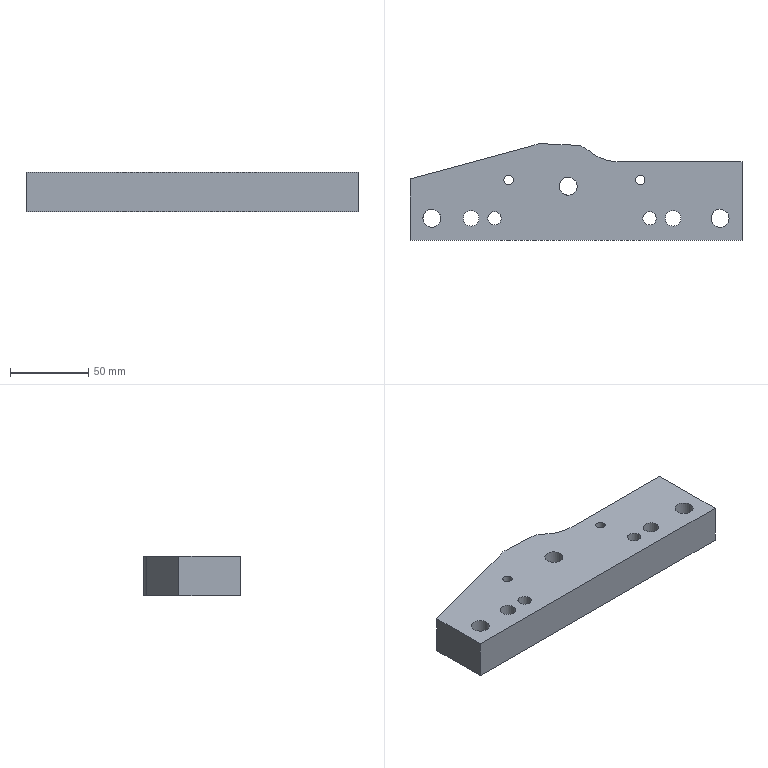Part | STEP file | lll_id3310_x_t | 1 solid | 30 faces | box 212 x 61.677 x 25 mm | volume 252902 mm3 | cylinder 14 | plane 13 | spline 3 | commonest cylinder face diameters 11.509 x3 18.007 x3 6 x2 8.505 x2 10 x2 12 x2
STEP:
#1=CARTESIAN_POINT('',(1787.,222.11,2.5));
#2=VERTEX_POINT('',#1);
#3=CARTESIAN_POINT('',(1787.,219.11,2.5));
#4=DIRECTION('',(0.,0.,-1.));
#5=DIRECTION('',(0.,1.,0.));
#6=AXIS2_PLACEMENT_3D('',#3,#4,#5);
#7=CIRCLE('',#6,3.);
#8=EDGE_CURVE('',#2,#2,#7,.T.);
#9=ORIENTED_EDGE('',*,*,#8,.F.);
#10=EDGE_LOOP('',(#9));
#11=FACE_BOUND('',#10,.T.);
#12=CARTESIAN_POINT('',(1871.,222.11,2.5));
#13=VERTEX_POINT('',#12);
#14=CARTESIAN_POINT('',(1871.,219.11,2.5));
#15=DIRECTION('',(0.,0.,-1.));
#16=DIRECTION('',(0.,1.,0.));
#17=AXIS2_PLACEMENT_3D('',#14,#15,#16);
#18=CIRCLE('',#17,3.);
#19=EDGE_CURVE('',#13,#13,#18,.T.);
#20=ORIENTED_EDGE('',*,*,#19,.F.);
#21=EDGE_LOOP('',(#20));
#22=FACE_BOUND('',#21,.T.);
#23=CARTESIAN_POINT('',(1784.,194.617,2.5));
#24=VERTEX_POINT('',#23);
#25=CARTESIAN_POINT('',(1778.,194.617,2.5));
#26=DIRECTION('',(0.,0.,1.));
#27=DIRECTION('',(1.,0.,0.));
#28=AXIS2_PLACEMENT_3D('',#25,#26,#27);
#29=CIRCLE('',#28,6.);
#30=EDGE_CURVE('',#24,#24,#29,.T.);
#31=ORIENTED_EDGE('',*,*,#30,.T.);
#32=EDGE_LOOP('',(#31));
#33=FACE_BOUND('',#32,.T.);
#34=CARTESIAN_POINT('',(1892.,189.617,2.5));
#35=VERTEX_POINT('',#34);
#36=CARTESIAN_POINT('',(1892.,194.617,2.5));
#37=DIRECTION('',(0.,0.,1.));
#38=DIRECTION('',(0.,-1.,0.));
#39=AXIS2_PLACEMENT_3D('',#36,#37,#38);
#40=CIRCLE('',#39,5.);
#41=EDGE_CURVE('',#35,#35,#40,.T.);
#42=ORIENTED_EDGE('',*,*,#41,.T.);
#43=EDGE_LOOP('',(#42));
#44=FACE_BOUND('',#43,.T.);
#45=CARTESIAN_POINT('',(1834.004,215.11,2.5));
#46=VERTEX_POINT('',#45);
#47=CARTESIAN_POINT('',(1825.,215.11,2.5));
#48=DIRECTION('',(0.,0.,-1.));
#49=DIRECTION('',(1.,0.,0.));
#50=AXIS2_PLACEMENT_3D('',#47,#48,#49);
#51=CIRCLE('',#50,9.004);
#52=EDGE_CURVE('',#46,#46,#51,.T.);
#53=ORIENTED_EDGE('',*,*,#52,.F.);
#54=EDGE_LOOP('',(#53));
#55=FACE_BOUND('',#54,.T.);
#56=CARTESIAN_POINT('',(1763.,189.617,2.5));
#57=VERTEX_POINT('',#56);
#58=CARTESIAN_POINT('',(1763.,194.617,2.5));
#59=DIRECTION('',(0.,0.,1.));
#60=DIRECTION('',(0.,-1.,0.));
#61=AXIS2_PLACEMENT_3D('',#58,#59,#60);
#62=CIRCLE('',#61,5.);
#63=EDGE_CURVE('',#57,#57,#62,.T.);
#64=ORIENTED_EDGE('',*,*,#63,.T.);
#65=EDGE_LOOP('',(#64));
#66=FACE_BOUND('',#65,.T.);
#67=CARTESIAN_POINT('',(1936.,180.617,2.5));
#68=VERTEX_POINT('',#67);
#69=CARTESIAN_POINT('',(1724.,180.617,2.5));
#70=VERTEX_POINT('',#69);
#71=CARTESIAN_POINT('',(12283.883,180.617,2.5));
#72=DIRECTION('',(-1.,0.,0.));
#73=VECTOR('',#72,1.);
#74=LINE('',#71,#73);
#75=EDGE_CURVE('',#68,#70,#74,.T.);
#76=ORIENTED_EDGE('',*,*,#75,.T.);
#77=CARTESIAN_POINT('',(1724.,219.798,2.5));
#78=VERTEX_POINT('',#77);
#79=CARTESIAN_POINT('',(1724.,-124.558,2.5));
#80=DIRECTION('',(0.,1.,0.));
#81=VECTOR('',#80,1.);
#82=LINE('',#79,#81);
#83=EDGE_CURVE('',#70,#78,#82,.T.);
#84=ORIENTED_EDGE('',*,*,#83,.T.);
#85=CARTESIAN_POINT('',(1799.668,240.307,2.5));
#86=VERTEX_POINT('',#85);
#87=CARTESIAN_POINT('',(14967.98,3809.511,2.5));
#88=DIRECTION('',(-0.9652,-0.2616,0.));
#89=VECTOR('',#88,1.);
#90=LINE('',#87,#89);
#91=EDGE_CURVE('',#86,#78,#90,.T.);
#92=ORIENTED_EDGE('',*,*,#91,.F.);
#93=CARTESIAN_POINT('',(1807.957,242.286,2.5));
#94=VERTEX_POINT('',#93);
#95=CARTESIAN_POINT('',(1799.668,240.307,2.5));
#96=CARTESIAN_POINT('',(1802.41,241.05,2.5));
#97=CARTESIAN_POINT('',(1805.12,242.415,2.5));
#98=CARTESIAN_POINT('',(1807.957,242.286,2.5));
#99=B_SPLINE_CURVE_WITH_KNOTS('',3,(#95,#96,#97,#98),.UNSPECIFIED.,.F.,.F.,(4,4),(0.,1.),.UNSPECIFIED.);
#100=EDGE_CURVE('',#86,#94,#99,.T.);
#101=ORIENTED_EDGE('',*,*,#100,.T.);
#102=CARTESIAN_POINT('',(1830.236,241.266,2.5));
#103=VERTEX_POINT('',#102);
#104=CARTESIAN_POINT('',(11646.576,-208.147,2.5));
#105=DIRECTION('',(0.999,-0.04573,0.));
#106=VECTOR('',#105,1.);
#107=LINE('',#104,#106);
#108=EDGE_CURVE('',#94,#103,#107,.T.);
#109=ORIENTED_EDGE('',*,*,#108,.T.);
#110=CARTESIAN_POINT('',(1837.708,238.136,2.5));
#111=VERTEX_POINT('',#110);
#112=CARTESIAN_POINT('',(1830.236,241.266,2.5));
#113=CARTESIAN_POINT('',(1830.337,241.261,2.5));
#114=CARTESIAN_POINT('',(1830.409,241.257,2.5));
#115=CARTESIAN_POINT('',(1830.582,241.245,2.5));
#116=CARTESIAN_POINT('',(1830.841,241.224,2.5));
#117=CARTESIAN_POINT('',(1831.442,241.157,2.5));
#118=CARTESIAN_POINT('',(1831.951,241.065,2.5));
#119=CARTESIAN_POINT('',(1832.959,240.837,2.5));
#120=CARTESIAN_POINT('',(1833.615,240.627,2.5));
#121=CARTESIAN_POINT('',(1834.882,240.096,2.5));
#122=CARTESIAN_POINT('',(1835.492,239.776,2.5));
#123=CARTESIAN_POINT('',(1836.361,239.218,2.5));
#124=CARTESIAN_POINT('',(1836.643,239.019,2.5));
#125=CARTESIAN_POINT('',(1837.053,238.702,2.5));
#126=CARTESIAN_POINT('',(1837.254,238.539,2.5));
#127=CARTESIAN_POINT('',(1837.451,238.369,2.5));
#128=CARTESIAN_POINT('',(1837.58,238.254,2.5));
#129=CARTESIAN_POINT('',(1837.634,238.206,2.5));
#130=CARTESIAN_POINT('',(1837.708,238.136,2.5));
#131=B_SPLINE_CURVE_WITH_KNOTS('',3,(#112,#113,#114,#115,#116,#117,#118,#119,#120,#121,#122,#123,#124,#125,#126,#127,#128,#129,#130),.UNSPECIFIED.,.F.,.F.,(4,2,1,1,2,2,2,2,1,2,4),(0.,0.03125,0.0625,0.125,0.25,0.5,0.75,0.875,0.9375,0.9688,1.),.UNSPECIFIED.);
#132=EDGE_CURVE('',#103,#111,#131,.T.);
#133=ORIENTED_EDGE('',*,*,#132,.T.);
#134=CARTESIAN_POINT('',(1856.885,230.617,2.5));
#135=VERTEX_POINT('',#134);
#136=CARTESIAN_POINT('',(1856.885,230.617,2.5));
#137=CARTESIAN_POINT('',(1855.125,230.617,2.5));
#138=CARTESIAN_POINT('',(1853.356,230.783,2.5));
#139=CARTESIAN_POINT('',(1849.901,231.439,2.5));
#140=CARTESIAN_POINT('',(1848.224,231.922,2.5));
#141=CARTESIAN_POINT('',(1844.948,233.206,2.5));
#142=CARTESIAN_POINT('',(1843.361,234.008,2.5));
#143=CARTESIAN_POINT('',(1841.14,235.403,2.5));
#144=CARTESIAN_POINT('',(1840.421,235.902,2.5));
#145=CARTESIAN_POINT('',(1839.378,236.701,2.5));
#146=CARTESIAN_POINT('',(1838.865,237.114,2.5));
#147=CARTESIAN_POINT('',(1838.365,237.546,2.5));
#148=CARTESIAN_POINT('',(1838.034,237.838,2.5));
#149=CARTESIAN_POINT('',(1837.859,237.997,2.5));
#150=CARTESIAN_POINT('',(1837.708,238.136,2.5));
#151=B_SPLINE_CURVE_WITH_KNOTS('',3,(#136,#137,#138,#139,#140,#141,#142,#143,#144,#145,#146,#147,#148,#149,#150),.UNSPECIFIED.,.F.,.F.,(4,2,2,2,2,1,2,4),(0.,0.25,0.5,0.75,0.875,0.9375,0.9688,1.),.UNSPECIFIED.);
#152=EDGE_CURVE('',#135,#111,#151,.T.);
#153=ORIENTED_EDGE('',*,*,#152,.F.);
#154=CARTESIAN_POINT('',(1936.,230.617,2.5));
#155=VERTEX_POINT('',#154);
#156=CARTESIAN_POINT('',(12283.883,230.617,2.5));
#157=DIRECTION('',(1.,0.,0.));
#158=VECTOR('',#157,1.);
#159=LINE('',#156,#158);
#160=EDGE_CURVE('',#135,#155,#159,.T.);
#161=ORIENTED_EDGE('',*,*,#160,.T.);
#162=CARTESIAN_POINT('',(1936.,-291.247,2.5));
#163=DIRECTION('',(0.,1.,0.));
#164=VECTOR('',#163,1.);
#165=LINE('',#162,#164);
#166=EDGE_CURVE('',#68,#155,#165,.T.);
#167=ORIENTED_EDGE('',*,*,#166,.F.);
#168=EDGE_LOOP('',(#76,#84,#92,#101,#109,#133,#153,#161,#167));
#169=FACE_BOUND('',#168,.T.);
#170=CARTESIAN_POINT('',(1747.004,194.617,2.5));
#171=VERTEX_POINT('',#170);
#172=CARTESIAN_POINT('',(1738.,194.617,2.5));
#173=DIRECTION('',(0.,0.,-1.));
#174=DIRECTION('',(1.,0.,0.));
#175=AXIS2_PLACEMENT_3D('',#172,#173,#174);
#176=CIRCLE('',#175,9.004);
#177=EDGE_CURVE('',#171,#171,#176,.T.);
#178=ORIENTED_EDGE('',*,*,#177,.F.);
#179=EDGE_LOOP('',(#178));
#180=FACE_BOUND('',#179,.T.);
#181=CARTESIAN_POINT('',(1931.004,194.617,2.5));
#182=VERTEX_POINT('',#181);
#183=CARTESIAN_POINT('',(1922.,194.617,2.5));
#184=DIRECTION('',(0.,0.,-1.));
#185=DIRECTION('',(1.,0.,0.));
#186=AXIS2_PLACEMENT_3D('',#183,#184,#185);
#187=CIRCLE('',#186,9.004);
#188=EDGE_CURVE('',#182,#182,#187,.T.);
#189=ORIENTED_EDGE('',*,*,#188,.F.);
#190=EDGE_LOOP('',(#189));
#191=FACE_BOUND('',#190,.T.);
#192=CARTESIAN_POINT('',(1883.,194.617,2.5));
#193=VERTEX_POINT('',#192);
#194=CARTESIAN_POINT('',(1877.,194.617,2.5));
#195=DIRECTION('',(0.,0.,1.));
#196=DIRECTION('',(1.,0.,0.));
#197=AXIS2_PLACEMENT_3D('',#194,#195,#196);
#198=CIRCLE('',#197,6.);
#199=EDGE_CURVE('',#193,#193,#198,.T.);
#200=ORIENTED_EDGE('',*,*,#199,.T.);
#201=EDGE_LOOP('',(#200));
#202=FACE_BOUND('',#201,.T.);
#203=CARTESIAN_POINT('',(12283.883,13712.286,2.5));
#204=DIRECTION('',(0.,0.,-1.));
#205=DIRECTION('',(1.,0.,0.));
#206=AXIS2_PLACEMENT_3D('',#203,#204,#205);
#207=PLANE('',#206);
#208=ADVANCED_FACE('',(#11,#22,#33,#44,#55,#66,#169,#180,#191,#202),#207,.T.);
#209=CARTESIAN_POINT('',(1724.,180.617,27.5));
#210=VERTEX_POINT('',#209);
#211=CARTESIAN_POINT('',(1724.,180.617,42.5));
#212=DIRECTION('',(0.,0.,1.));
#213=VECTOR('',#212,1.);
#214=LINE('',#211,#213);
#215=EDGE_CURVE('',#70,#210,#214,.T.);
#216=ORIENTED_EDGE('',*,*,#215,.F.);
#217=ORIENTED_EDGE('',*,*,#75,.F.);
#218=CARTESIAN_POINT('',(1936.,180.617,27.5));
#219=VERTEX_POINT('',#218);
#220=CARTESIAN_POINT('',(1936.,180.617,39.614));
#221=DIRECTION('',(0.,0.,1.));
#222=VECTOR('',#221,1.);
#223=LINE('',#220,#222);
#224=EDGE_CURVE('',#68,#219,#223,.T.);
#225=ORIENTED_EDGE('',*,*,#224,.T.);
#226=CARTESIAN_POINT('',(1834.,180.617,27.5));
#227=DIRECTION('',(1.,0.,0.));
#228=VECTOR('',#227,1.);
#229=LINE('',#226,#228);
#230=EDGE_CURVE('',#210,#219,#229,.T.);
#231=ORIENTED_EDGE('',*,*,#230,.F.);
#232=EDGE_LOOP('',(#216,#217,#225,#231));
#233=FACE_OUTER_BOUND('',#232,.T.);
#234=CARTESIAN_POINT('',(1900.443,180.617,34.5));
#235=DIRECTION('',(0.,1.,0.));
#236=DIRECTION('',(0.,0.,1.));
#237=AXIS2_PLACEMENT_3D('',#234,#235,#236);
#238=PLANE('',#237);
#239=ADVANCED_FACE('',(#233),#238,.F.);
#240=ORIENTED_EDGE('',*,*,#224,.F.);
#241=ORIENTED_EDGE('',*,*,#166,.T.);
#242=CARTESIAN_POINT('',(1936.,230.617,27.5));
#243=VERTEX_POINT('',#242);
#244=CARTESIAN_POINT('',(1936.,230.617,39.614));
#245=DIRECTION('',(0.,0.,-1.));
#246=VECTOR('',#245,1.);
#247=LINE('',#244,#246);
#248=EDGE_CURVE('',#243,#155,#247,.T.);
#249=ORIENTED_EDGE('',*,*,#248,.F.);
#250=CARTESIAN_POINT('',(1936.,-0.5,27.5));
#251=DIRECTION('',(0.,1.,0.));
#252=VECTOR('',#251,1.);
#253=LINE('',#250,#252);
#254=EDGE_CURVE('',#219,#243,#253,.T.);
#255=ORIENTED_EDGE('',*,*,#254,.F.);
#256=EDGE_LOOP('',(#240,#241,#249,#255));
#257=FACE_OUTER_BOUND('',#256,.T.);
#258=CARTESIAN_POINT('',(1936.,-291.247,39.614));
#259=DIRECTION('',(1.,0.,0.));
#260=DIRECTION('',(0.,0.,1.));
#261=AXIS2_PLACEMENT_3D('',#258,#259,#260);
#262=PLANE('',#261);
#263=ADVANCED_FACE('',(#257),#262,.T.);
#264=CARTESIAN_POINT('',(1724.,219.798,27.5));
#265=VERTEX_POINT('',#264);
#266=CARTESIAN_POINT('',(1724.,219.798,-15.5));
#267=DIRECTION('',(0.,0.,-1.));
#268=VECTOR('',#267,1.);
#269=LINE('',#266,#268);
#270=EDGE_CURVE('',#265,#78,#269,.T.);
#271=ORIENTED_EDGE('',*,*,#270,.T.);
#272=ORIENTED_EDGE('',*,*,#83,.F.);
#273=ORIENTED_EDGE('',*,*,#215,.T.);
#274=CARTESIAN_POINT('',(1724.,-124.558,27.5));
#275=DIRECTION('',(0.,1.,0.));
#276=VECTOR('',#275,1.);
#277=LINE('',#274,#276);
#278=EDGE_CURVE('',#210,#265,#277,.T.);
#279=ORIENTED_EDGE('',*,*,#278,.T.);
#280=EDGE_LOOP('',(#271,#272,#273,#279));
#281=FACE_OUTER_BOUND('',#280,.T.);
#282=CARTESIAN_POINT('',(1724.,-124.558,42.5));
#283=DIRECTION('',(1.,0.,0.));
#284=DIRECTION('',(0.,0.,1.));
#285=AXIS2_PLACEMENT_3D('',#282,#283,#284);
#286=PLANE('',#285);
#287=ADVANCED_FACE('',(#281),#286,.F.);
#288=CARTESIAN_POINT('',(1799.668,240.307,27.5));
#289=VERTEX_POINT('',#288);
#290=CARTESIAN_POINT('',(1799.668,240.307,27.5));
#291=DIRECTION('',(-0.9652,-0.2616,0.));
#292=VECTOR('',#291,1.);
#293=LINE('',#290,#292);
#294=EDGE_CURVE('',#289,#265,#293,.T.);
#295=ORIENTED_EDGE('',*,*,#294,.F.);
#296=CARTESIAN_POINT('',(1799.668,240.307,59.5));
#297=DIRECTION('',(0.,0.,1.));
#298=VECTOR('',#297,1.);
#299=LINE('',#296,#298);
#300=EDGE_CURVE('',#86,#289,#299,.T.);
#301=ORIENTED_EDGE('',*,*,#300,.F.);
#302=ORIENTED_EDGE('',*,*,#91,.T.);
#303=ORIENTED_EDGE('',*,*,#270,.F.);
#304=EDGE_LOOP('',(#295,#301,#302,#303));
#305=FACE_OUTER_BOUND('',#304,.T.);
#306=CARTESIAN_POINT('',(1799.668,240.307,-15.5));
#307=DIRECTION('',(-0.2616,0.9652,0.));
#308=DIRECTION('',(-0.9652,-0.2616,0.));
#309=AXIS2_PLACEMENT_3D('',#306,#307,#308);
#310=PLANE('',#309);
#311=ADVANCED_FACE('',(#305),#310,.T.);
#312=ORIENTED_EDGE('',*,*,#248,.T.);
#313=ORIENTED_EDGE('',*,*,#160,.F.);
#314=CARTESIAN_POINT('',(1856.885,230.617,27.5));
#315=VERTEX_POINT('',#314);
#316=CARTESIAN_POINT('',(1856.885,230.617,-15.5));
#317=DIRECTION('',(0.,0.,-1.));
#318=VECTOR('',#317,1.);
#319=LINE('',#316,#318);
#320=EDGE_CURVE('',#315,#135,#319,.T.);
#321=ORIENTED_EDGE('',*,*,#320,.F.);
#322=CARTESIAN_POINT('',(1834.,230.617,27.5));
#323=DIRECTION('',(-1.,0.,0.));
#324=VECTOR('',#323,1.);
#325=LINE('',#322,#324);
#326=EDGE_CURVE('',#243,#315,#325,.T.);
#327=ORIENTED_EDGE('',*,*,#326,.F.);
#328=EDGE_LOOP('',(#312,#313,#321,#327));
#329=FACE_OUTER_BOUND('',#328,.T.);
#330=CARTESIAN_POINT('',(1856.885,230.617,-15.5));
#331=DIRECTION('',(0.,-1.,0.));
#332=DIRECTION('',(0.,0.,1.));
#333=AXIS2_PLACEMENT_3D('',#330,#331,#332);
#334=PLANE('',#333);
#335=ADVANCED_FACE('',(#329),#334,.F.);
#336=ORIENTED_EDGE('',*,*,#320,.T.);
#337=ORIENTED_EDGE('',*,*,#152,.T.);
#338=CARTESIAN_POINT('',(1837.708,238.136,27.5));
#339=VERTEX_POINT('',#338);
#340=CARTESIAN_POINT('',(1837.708,238.136,-15.5));
#341=DIRECTION('',(0.,0.,-1.));
#342=VECTOR('',#341,1.);
#343=LINE('',#340,#342);
#344=EDGE_CURVE('',#339,#111,#343,.T.);
#345=ORIENTED_EDGE('',*,*,#344,.F.);
#346=CARTESIAN_POINT('',(1856.885,230.617,27.5));
#347=CARTESIAN_POINT('',(1855.125,230.617,27.5));
#348=CARTESIAN_POINT('',(1853.356,230.783,27.5));
#349=CARTESIAN_POINT('',(1849.901,231.439,27.5));
#350=CARTESIAN_POINT('',(1848.224,231.922,27.5));
#351=CARTESIAN_POINT('',(1844.948,233.206,27.5));
#352=CARTESIAN_POINT('',(1843.361,234.008,27.5));
#353=CARTESIAN_POINT('',(1841.14,235.403,27.5));
#354=CARTESIAN_POINT('',(1840.421,235.902,27.5));
#355=CARTESIAN_POINT('',(1839.378,236.701,27.5));
#356=CARTESIAN_POINT('',(1838.865,237.114,27.5));
#357=CARTESIAN_POINT('',(1838.365,237.546,27.5));
#358=CARTESIAN_POINT('',(1838.034,237.838,27.5));
#359=CARTESIAN_POINT('',(1837.859,237.997,27.5));
#360=CARTESIAN_POINT('',(1837.708,238.136,27.5));
#361=B_SPLINE_CURVE_WITH_KNOTS('',3,(#346,#347,#348,#349,#350,#351,#352,#353,#354,#355,#356,#357,#358,#359,#360),.UNSPECIFIED.,.F.,.F.,(4,2,2,2,2,1,2,4),(0.,0.25,0.5,0.75,0.875,0.9375,0.9688,1.),.UNSPECIFIED.);
#362=EDGE_CURVE('',#315,#339,#361,.T.);
#363=ORIENTED_EDGE('',*,*,#362,.F.);
#364=EDGE_LOOP('',(#336,#337,#345,#363));
#365=FACE_OUTER_BOUND('',#364,.T.);
#366=CARTESIAN_POINT('',(1856.885,230.617,2.5));
#367=CARTESIAN_POINT('',(1856.885,230.617,27.5));
#368=CARTESIAN_POINT('',(1855.125,230.617,2.5));
#369=CARTESIAN_POINT('',(1855.125,230.617,27.5));
#370=CARTESIAN_POINT('',(1853.356,230.783,2.5));
#371=CARTESIAN_POINT('',(1853.356,230.783,27.5));
#372=CARTESIAN_POINT('',(1849.901,231.439,2.5));
#373=CARTESIAN_POINT('',(1849.901,231.439,27.5));
#374=CARTESIAN_POINT('',(1848.224,231.922,2.5));
#375=CARTESIAN_POINT('',(1848.224,231.922,27.5));
#376=CARTESIAN_POINT('',(1844.948,233.206,2.5));
#377=CARTESIAN_POINT('',(1844.948,233.206,27.5));
#378=CARTESIAN_POINT('',(1843.361,234.008,2.5));
#379=CARTESIAN_POINT('',(1843.361,234.008,27.5));
#380=CARTESIAN_POINT('',(1841.14,235.403,2.5));
#381=CARTESIAN_POINT('',(1841.14,235.403,27.5));
#382=CARTESIAN_POINT('',(1840.421,235.902,2.5));
#383=CARTESIAN_POINT('',(1840.421,235.902,27.5));
#384=CARTESIAN_POINT('',(1839.378,236.701,2.5));
#385=CARTESIAN_POINT('',(1839.378,236.701,27.5));
#386=CARTESIAN_POINT('',(1838.865,237.114,2.5));
#387=CARTESIAN_POINT('',(1838.865,237.114,27.5));
#388=CARTESIAN_POINT('',(1838.365,237.546,2.5));
#389=CARTESIAN_POINT('',(1838.365,237.546,27.5));
#390=CARTESIAN_POINT('',(1838.034,237.838,2.5));
#391=CARTESIAN_POINT('',(1838.034,237.838,27.5));
#392=CARTESIAN_POINT('',(1837.859,237.997,2.5));
#393=CARTESIAN_POINT('',(1837.859,237.997,27.5));
#394=CARTESIAN_POINT('',(1837.708,238.136,2.5));
#395=CARTESIAN_POINT('',(1837.708,238.136,27.5));
#396=B_SPLINE_SURFACE_WITH_KNOTS('',3,1,((#366,#367),(#368,#369),(#370,#371),(#372,#373),(#374,#375),(#376,#377),(#378,#379),(#380,#381),(#382,#383),(#384,#385),(#386,#387),(#388,#389),(#390,#391),(#392,#393),(#394,#395)),.UNSPECIFIED.,.F.,.F.,.F.,(4,2,2,2,2,1,2,4),(2,2),(0.,0.25,0.5,0.75,0.875,0.9375,0.9688,1.),(0.,1.),.UNSPECIFIED.);
#397=ADVANCED_FACE('',(#365),#396,.T.);
#398=ORIENTED_EDGE('',*,*,#344,.T.);
#399=ORIENTED_EDGE('',*,*,#132,.F.);
#400=CARTESIAN_POINT('',(1830.236,241.266,27.5));
#401=VERTEX_POINT('',#400);
#402=CARTESIAN_POINT('',(1830.236,241.266,-15.5));
#403=DIRECTION('',(0.,0.,-1.));
#404=VECTOR('',#403,1.);
#405=LINE('',#402,#404);
#406=EDGE_CURVE('',#401,#103,#405,.T.);
#407=ORIENTED_EDGE('',*,*,#406,.F.);
#408=CARTESIAN_POINT('',(1830.236,241.266,27.5));
#409=CARTESIAN_POINT('',(1830.337,241.261,27.5));
#410=CARTESIAN_POINT('',(1830.409,241.257,27.5));
#411=CARTESIAN_POINT('',(1830.582,241.245,27.5));
#412=CARTESIAN_POINT('',(1830.841,241.224,27.5));
#413=CARTESIAN_POINT('',(1831.442,241.157,27.5));
#414=CARTESIAN_POINT('',(1831.951,241.065,27.5));
#415=CARTESIAN_POINT('',(1832.959,240.837,27.5));
#416=CARTESIAN_POINT('',(1833.615,240.627,27.5));
#417=CARTESIAN_POINT('',(1834.882,240.096,27.5));
#418=CARTESIAN_POINT('',(1835.492,239.776,27.5));
#419=CARTESIAN_POINT('',(1836.361,239.218,27.5));
#420=CARTESIAN_POINT('',(1836.643,239.019,27.5));
#421=CARTESIAN_POINT('',(1837.053,238.702,27.5));
#422=CARTESIAN_POINT('',(1837.254,238.539,27.5));
#423=CARTESIAN_POINT('',(1837.451,238.369,27.5));
#424=CARTESIAN_POINT('',(1837.58,238.254,27.5));
#425=CARTESIAN_POINT('',(1837.634,238.206,27.5));
#426=CARTESIAN_POINT('',(1837.708,238.136,27.5));
#427=B_SPLINE_CURVE_WITH_KNOTS('',3,(#408,#409,#410,#411,#412,#413,#414,#415,#416,#417,#418,#419,#420,#421,#422,#423,#424,#425,#426),.UNSPECIFIED.,.F.,.F.,(4,2,1,1,2,2,2,2,1,2,4),(0.,0.03125,0.0625,0.125,0.25,0.5,0.75,0.875,0.9375,0.9688,1.),.UNSPECIFIED.);
#428=EDGE_CURVE('',#401,#339,#427,.T.);
#429=ORIENTED_EDGE('',*,*,#428,.T.);
#430=EDGE_LOOP('',(#398,#399,#407,#429));
#431=FACE_OUTER_BOUND('',#430,.T.);
#432=CARTESIAN_POINT('',(1837.708,238.136,2.5));
#433=CARTESIAN_POINT('',(1837.708,238.136,27.5));
#434=CARTESIAN_POINT('',(1837.634,238.206,2.5));
#435=CARTESIAN_POINT('',(1837.634,238.206,27.5));
#436=CARTESIAN_POINT('',(1837.58,238.254,2.5));
#437=CARTESIAN_POINT('',(1837.58,238.254,27.5));
#438=CARTESIAN_POINT('',(1837.451,238.369,2.5));
#439=CARTESIAN_POINT('',(1837.451,238.369,27.5));
#440=CARTESIAN_POINT('',(1837.254,238.539,2.5));
#441=CARTESIAN_POINT('',(1837.254,238.539,27.5));
#442=CARTESIAN_POINT('',(1837.053,238.702,2.5));
#443=CARTESIAN_POINT('',(1837.053,238.702,27.5));
#444=CARTESIAN_POINT('',(1836.643,239.019,2.5));
#445=CARTESIAN_POINT('',(1836.643,239.019,27.5));
#446=CARTESIAN_POINT('',(1836.361,239.218,2.5));
#447=CARTESIAN_POINT('',(1836.361,239.218,27.5));
#448=CARTESIAN_POINT('',(1835.492,239.776,2.5));
#449=CARTESIAN_POINT('',(1835.492,239.776,27.5));
#450=CARTESIAN_POINT('',(1834.882,240.096,2.5));
#451=CARTESIAN_POINT('',(1834.882,240.096,27.5));
#452=CARTESIAN_POINT('',(1833.615,240.627,2.5));
#453=CARTESIAN_POINT('',(1833.615,240.627,27.5));
#454=CARTESIAN_POINT('',(1832.959,240.837,2.5));
#455=CARTESIAN_POINT('',(1832.959,240.837,27.5));
#456=CARTESIAN_POINT('',(1831.951,241.065,2.5));
#457=CARTESIAN_POINT('',(1831.951,241.065,27.5));
#458=CARTESIAN_POINT('',(1831.442,241.157,2.5));
#459=CARTESIAN_POINT('',(1831.442,241.157,27.5));
#460=CARTESIAN_POINT('',(1830.841,241.224,2.5));
#461=CARTESIAN_POINT('',(1830.841,241.224,27.5));
#462=CARTESIAN_POINT('',(1830.582,241.245,2.5));
#463=CARTESIAN_POINT('',(1830.582,241.245,27.5));
#464=CARTESIAN_POINT('',(1830.409,241.257,2.5));
#465=CARTESIAN_POINT('',(1830.409,241.257,27.5));
#466=CARTESIAN_POINT('',(1830.337,241.261,2.5));
#467=CARTESIAN_POINT('',(1830.337,241.261,27.5));
#468=CARTESIAN_POINT('',(1830.236,241.266,2.5));
#469=CARTESIAN_POINT('',(1830.236,241.266,27.5));
#470=B_SPLINE_SURFACE_WITH_KNOTS('',3,1,((#432,#433),(#434,#435),(#436,#437),(#438,#439),(#440,#441),(#442,#443),(#444,#445),(#446,#447),(#448,#449),(#450,#451),(#452,#453),(#454,#455),(#456,#457),(#458,#459),(#460,#461),(#462,#463),(#464,#465),(#466,#467),(#468,#469)),.UNSPECIFIED.,.F.,.F.,.F.,(4,2,1,2,2,2,2,1,1,2,4),(2,2),(0.,0.03125,0.0625,0.125,0.25,0.5,0.75,0.875,0.9375,0.9687,1.),(0.,1.),.UNSPECIFIED.);
#471=ADVANCED_FACE('',(#431),#470,.T.);
#472=ORIENTED_EDGE('',*,*,#406,.T.);
#473=ORIENTED_EDGE('',*,*,#108,.F.);
#474=CARTESIAN_POINT('',(1807.957,242.286,27.5));
#475=VERTEX_POINT('',#474);
#476=CARTESIAN_POINT('',(1807.957,242.286,-15.5));
#477=DIRECTION('',(0.,0.,1.));
#478=VECTOR('',#477,1.);
#479=LINE('',#476,#478);
#480=EDGE_CURVE('',#94,#475,#479,.T.);
#481=ORIENTED_EDGE('',*,*,#480,.T.);
#482=CARTESIAN_POINT('',(1807.957,242.286,27.5));
#483=DIRECTION('',(0.999,-0.04573,0.));
#484=VECTOR('',#483,1.);
#485=LINE('',#482,#484);
#486=EDGE_CURVE('',#475,#401,#485,.T.);
#487=ORIENTED_EDGE('',*,*,#486,.T.);
#488=EDGE_LOOP('',(#472,#473,#481,#487));
#489=FACE_OUTER_BOUND('',#488,.T.);
#490=CARTESIAN_POINT('',(1807.957,242.286,-15.5));
#491=DIRECTION('',(-0.04573,-0.999,0.));
#492=DIRECTION('',(0.999,-0.04573,0.));
#493=AXIS2_PLACEMENT_3D('',#490,#491,#492);
#494=PLANE('',#493);
#495=ADVANCED_FACE('',(#489),#494,.F.);
#496=ORIENTED_EDGE('',*,*,#480,.F.);
#497=ORIENTED_EDGE('',*,*,#100,.F.);
#498=ORIENTED_EDGE('',*,*,#300,.T.);
#499=CARTESIAN_POINT('',(1799.668,240.307,27.5));
#500=CARTESIAN_POINT('',(1802.41,241.05,27.5));
#501=CARTESIAN_POINT('',(1805.12,242.415,27.5));
#502=CARTESIAN_POINT('',(1807.957,242.286,27.5));
#503=B_SPLINE_CURVE_WITH_KNOTS('',3,(#499,#500,#501,#502),.UNSPECIFIED.,.F.,.F.,(4,4),(0.,1.),.UNSPECIFIED.);
#504=EDGE_CURVE('',#289,#475,#503,.T.);
#505=ORIENTED_EDGE('',*,*,#504,.T.);
#506=EDGE_LOOP('',(#496,#497,#498,#505));
#507=FACE_OUTER_BOUND('',#506,.T.);
#508=CARTESIAN_POINT('',(1807.957,242.286,-15.5));
#509=CARTESIAN_POINT('',(1805.12,242.415,-15.5));
#510=CARTESIAN_POINT('',(1802.41,241.05,-15.5));
#511=CARTESIAN_POINT('',(1799.668,240.307,-15.5));
#512=CARTESIAN_POINT('',(1807.957,242.286,134.5));
#513=CARTESIAN_POINT('',(1805.12,242.415,134.5));
#514=CARTESIAN_POINT('',(1802.41,241.05,134.5));
#515=CARTESIAN_POINT('',(1799.668,240.307,134.5));
#516=B_SPLINE_SURFACE_WITH_KNOTS('',1,3,((#508,#509,#510,#511),(#512,#513,#514,#515)),.UNSPECIFIED.,.F.,.F.,.F.,(2,2),(4,4),(0.,1.),(0.,1.),.UNSPECIFIED.);
#517=ADVANCED_FACE('',(#507),#516,.F.);
#518=CARTESIAN_POINT('',(1787.,222.11,27.5));
#519=VERTEX_POINT('',#518);
#520=CARTESIAN_POINT('',(1787.,219.11,27.5));
#521=DIRECTION('',(0.,0.,-1.));
#522=DIRECTION('',(0.,1.,0.));
#523=AXIS2_PLACEMENT_3D('',#520,#521,#522);
#524=CIRCLE('',#523,3.);
#525=EDGE_CURVE('',#519,#519,#524,.T.);
#526=ORIENTED_EDGE('',*,*,#525,.T.);
#527=EDGE_LOOP('',(#526));
#528=FACE_BOUND('',#527,.T.);
#529=CARTESIAN_POINT('',(1871.,222.11,27.5));
#530=VERTEX_POINT('',#529);
#531=CARTESIAN_POINT('',(1871.,219.11,27.5));
#532=DIRECTION('',(0.,0.,-1.));
#533=DIRECTION('',(0.,1.,0.));
#534=AXIS2_PLACEMENT_3D('',#531,#532,#533);
#535=CIRCLE('',#534,3.);
#536=EDGE_CURVE('',#530,#530,#535,.T.);
#537=ORIENTED_EDGE('',*,*,#536,.T.);
#538=EDGE_LOOP('',(#537));
#539=FACE_BOUND('',#538,.T.);
#540=CARTESIAN_POINT('',(1877.,198.869,27.5));
#541=VERTEX_POINT('',#540);
#542=CARTESIAN_POINT('',(1877.,194.617,27.5));
#543=DIRECTION('',(0.,0.,1.));
#544=DIRECTION('',(0.,1.,0.));
#545=AXIS2_PLACEMENT_3D('',#542,#543,#544);
#546=CIRCLE('',#545,4.253);
#547=EDGE_CURVE('',#541,#541,#546,.T.);
#548=ORIENTED_EDGE('',*,*,#547,.F.);
#549=EDGE_LOOP('',(#548));
#550=FACE_BOUND('',#549,.T.);
#551=CARTESIAN_POINT('',(1892.,199.617,27.5));
#552=VERTEX_POINT('',#551);
#553=CARTESIAN_POINT('',(1892.,194.617,27.5));
#554=DIRECTION('',(0.,0.,1.));
#555=DIRECTION('',(0.,1.,0.));
#556=AXIS2_PLACEMENT_3D('',#553,#554,#555);
#557=CIRCLE('',#556,5.);
#558=EDGE_CURVE('',#552,#552,#557,.T.);
#559=ORIENTED_EDGE('',*,*,#558,.F.);
#560=EDGE_LOOP('',(#559));
#561=FACE_BOUND('',#560,.T.);
#562=CARTESIAN_POINT('',(1922.,200.371,27.5));
#563=VERTEX_POINT('',#562);
#564=CARTESIAN_POINT('',(1922.,194.617,27.5));
#565=DIRECTION('',(0.,0.,1.));
#566=DIRECTION('',(0.,1.,0.));
#567=AXIS2_PLACEMENT_3D('',#564,#565,#566);
#568=CIRCLE('',#567,5.755);
#569=EDGE_CURVE('',#563,#563,#568,.T.);
#570=ORIENTED_EDGE('',*,*,#569,.F.);
#571=EDGE_LOOP('',(#570));
#572=FACE_BOUND('',#571,.T.);
#573=CARTESIAN_POINT('',(1825.,220.865,27.5));
#574=VERTEX_POINT('',#573);
#575=CARTESIAN_POINT('',(1825.,215.11,27.5));
#576=DIRECTION('',(0.,0.,1.));
#577=DIRECTION('',(0.,1.,0.));
#578=AXIS2_PLACEMENT_3D('',#575,#576,#577);
#579=CIRCLE('',#578,5.755);
#580=EDGE_CURVE('',#574,#574,#579,.T.);
#581=ORIENTED_EDGE('',*,*,#580,.F.);
#582=EDGE_LOOP('',(#581));
#583=FACE_BOUND('',#582,.T.);
#584=CARTESIAN_POINT('',(1778.,198.869,27.5));
#585=VERTEX_POINT('',#584);
#586=CARTESIAN_POINT('',(1778.,194.617,27.5));
#587=DIRECTION('',(0.,0.,1.));
#588=DIRECTION('',(0.,1.,0.));
#589=AXIS2_PLACEMENT_3D('',#586,#587,#588);
#590=CIRCLE('',#589,4.253);
#591=EDGE_CURVE('',#585,#585,#590,.T.);
#592=ORIENTED_EDGE('',*,*,#591,.F.);
#593=EDGE_LOOP('',(#592));
#594=FACE_BOUND('',#593,.T.);
#595=CARTESIAN_POINT('',(1763.,199.617,27.5));
#596=VERTEX_POINT('',#595);
#597=CARTESIAN_POINT('',(1763.,194.617,27.5));
#598=DIRECTION('',(0.,0.,1.));
#599=DIRECTION('',(0.,1.,0.));
#600=AXIS2_PLACEMENT_3D('',#597,#598,#599);
#601=CIRCLE('',#600,5.);
#602=EDGE_CURVE('',#596,#596,#601,.T.);
#603=ORIENTED_EDGE('',*,*,#602,.F.);
#604=EDGE_LOOP('',(#603));
#605=FACE_BOUND('',#604,.T.);
#606=CARTESIAN_POINT('',(1738.,200.371,27.5));
#607=VERTEX_POINT('',#606);
#608=CARTESIAN_POINT('',(1738.,194.617,27.5));
#609=DIRECTION('',(0.,0.,1.));
#610=DIRECTION('',(0.,1.,0.));
#611=AXIS2_PLACEMENT_3D('',#608,#609,#610);
#612=CIRCLE('',#611,5.755);
#613=EDGE_CURVE('',#607,#607,#612,.T.);
#614=ORIENTED_EDGE('',*,*,#613,.F.);
#615=EDGE_LOOP('',(#614));
#616=FACE_BOUND('',#615,.T.);
#617=ORIENTED_EDGE('',*,*,#486,.F.);
#618=ORIENTED_EDGE('',*,*,#504,.F.);
#619=ORIENTED_EDGE('',*,*,#294,.T.);
#620=ORIENTED_EDGE('',*,*,#278,.F.);
#621=ORIENTED_EDGE('',*,*,#230,.T.);
#622=ORIENTED_EDGE('',*,*,#254,.T.);
#623=ORIENTED_EDGE('',*,*,#326,.T.);
#624=ORIENTED_EDGE('',*,*,#362,.T.);
#625=ORIENTED_EDGE('',*,*,#428,.F.);
#626=EDGE_LOOP('',(#617,#618,#619,#620,#621,#622,#623,#624,#625));
#627=FACE_BOUND('',#626,.T.);
#628=CARTESIAN_POINT('',(1834.,-0.5,27.5));
#629=DIRECTION('',(0.,0.,-1.));
#630=DIRECTION('',(0.,1.,0.));
#631=AXIS2_PLACEMENT_3D('',#628,#629,#630);
#632=PLANE('',#631);
#633=ADVANCED_FACE('',(#528,#539,#550,#561,#572,#583,#594,#605,#616,#627),#632,.F.);
#634=CARTESIAN_POINT('',(1743.755,194.617,15.5));
#635=VERTEX_POINT('',#634);
#636=CARTESIAN_POINT('',(1738.,194.617,15.5));
#637=DIRECTION('',(0.,0.,-1.));
#638=DIRECTION('',(1.,0.,0.));
#639=AXIS2_PLACEMENT_3D('',#636,#637,#638);
#640=CIRCLE('',#639,5.755);
#641=EDGE_CURVE('',#635,#635,#640,.T.);
#642=ORIENTED_EDGE('',*,*,#641,.T.);
#643=EDGE_LOOP('',(#642));
#644=FACE_BOUND('',#643,.T.);
#645=ORIENTED_EDGE('',*,*,#613,.T.);
#646=EDGE_LOOP('',(#645));
#647=FACE_BOUND('',#646,.T.);
#648=CARTESIAN_POINT('',(1738.,194.617,-2.5));
#649=DIRECTION('',(0.,0.,1.));
#650=DIRECTION('',(1.,0.,0.));
#651=AXIS2_PLACEMENT_3D('',#648,#649,#650);
#652=CYLINDRICAL_SURFACE('',#651,5.755);
#653=ADVANCED_FACE('',(#644,#647),#652,.F.);
#654=ORIENTED_EDGE('',*,*,#641,.F.);
#655=EDGE_LOOP('',(#654));
#656=FACE_BOUND('',#655,.T.);
#657=CARTESIAN_POINT('',(1747.004,194.617,15.5));
#658=VERTEX_POINT('',#657);
#659=CARTESIAN_POINT('',(1738.,194.617,15.5));
#660=DIRECTION('',(0.,0.,-1.));
#661=DIRECTION('',(1.,0.,0.));
#662=AXIS2_PLACEMENT_3D('',#659,#660,#661);
#663=CIRCLE('',#662,9.004);
#664=EDGE_CURVE('',#658,#658,#663,.T.);
#665=ORIENTED_EDGE('',*,*,#664,.T.);
#666=EDGE_LOOP('',(#665));
#667=FACE_BOUND('',#666,.T.);
#668=CARTESIAN_POINT('',(1738.,194.617,15.5));
#669=DIRECTION('',(0.,0.,1.));
#670=DIRECTION('',(1.,0.,0.));
#671=AXIS2_PLACEMENT_3D('',#668,#669,#670);
#672=PLANE('',#671);
#673=ADVANCED_FACE('',(#656,#667),#672,.F.);
#674=ORIENTED_EDGE('',*,*,#664,.F.);
#675=EDGE_LOOP('',(#674));
#676=FACE_BOUND('',#675,.T.);
#677=ORIENTED_EDGE('',*,*,#177,.T.);
#678=EDGE_LOOP('',(#677));
#679=FACE_BOUND('',#678,.T.);
#680=CARTESIAN_POINT('',(1738.,194.617,2.5));
#681=DIRECTION('',(0.,0.,1.));
#682=DIRECTION('',(1.,0.,0.));
#683=AXIS2_PLACEMENT_3D('',#680,#681,#682);
#684=CYLINDRICAL_SURFACE('',#683,9.004);
#685=ADVANCED_FACE('',(#676,#679),#684,.F.);
#686=ORIENTED_EDGE('',*,*,#63,.F.);
#687=EDGE_LOOP('',(#686));
#688=FACE_BOUND('',#687,.T.);
#689=ORIENTED_EDGE('',*,*,#602,.T.);
#690=EDGE_LOOP('',(#689));
#691=FACE_BOUND('',#690,.T.);
#692=CARTESIAN_POINT('',(1763.,194.617,-2.5));
#693=DIRECTION('',(0.,0.,1.));
#694=DIRECTION('',(-1.,0.,0.));
#695=AXIS2_PLACEMENT_3D('',#692,#693,#694);
#696=CYLINDRICAL_SURFACE('',#695,5.);
#697=ADVANCED_FACE('',(#688,#691),#696,.F.);
#698=CARTESIAN_POINT('',(1778.,190.364,7.5));
#699=VERTEX_POINT('',#698);
#700=CARTESIAN_POINT('',(1778.,194.617,7.5));
#701=DIRECTION('',(0.,0.,-1.));
#702=DIRECTION('',(0.,-1.,0.));
#703=AXIS2_PLACEMENT_3D('',#700,#701,#702);
#704=CIRCLE('',#703,4.253);
#705=EDGE_CURVE('',#699,#699,#704,.T.);
#706=ORIENTED_EDGE('',*,*,#705,.T.);
#707=EDGE_LOOP('',(#706));
#708=FACE_BOUND('',#707,.T.);
#709=ORIENTED_EDGE('',*,*,#591,.T.);
#710=EDGE_LOOP('',(#709));
#711=FACE_BOUND('',#710,.T.);
#712=CARTESIAN_POINT('',(1778.,194.617,-2.5));
#713=DIRECTION('',(0.,0.,1.));
#714=DIRECTION('',(1.,0.,0.));
#715=AXIS2_PLACEMENT_3D('',#712,#713,#714);
#716=CYLINDRICAL_SURFACE('',#715,4.253);
#717=ADVANCED_FACE('',(#708,#711),#716,.F.);
#718=CARTESIAN_POINT('',(1830.755,215.11,15.5));
#719=VERTEX_POINT('',#718);
#720=CARTESIAN_POINT('',(1825.,215.11,15.5));
#721=DIRECTION('',(0.,0.,-1.));
#722=DIRECTION('',(1.,0.,0.));
#723=AXIS2_PLACEMENT_3D('',#720,#721,#722);
#724=CIRCLE('',#723,5.755);
#725=EDGE_CURVE('',#719,#719,#724,.T.);
#726=ORIENTED_EDGE('',*,*,#725,.T.);
#727=EDGE_LOOP('',(#726));
#728=FACE_BOUND('',#727,.T.);
#729=ORIENTED_EDGE('',*,*,#580,.T.);
#730=EDGE_LOOP('',(#729));
#731=FACE_BOUND('',#730,.T.);
#732=CARTESIAN_POINT('',(1825.,215.11,-2.5));
#733=DIRECTION('',(0.,0.,1.));
#734=DIRECTION('',(1.,0.,0.));
#735=AXIS2_PLACEMENT_3D('',#732,#733,#734);
#736=CYLINDRICAL_SURFACE('',#735,5.755);
#737=ADVANCED_FACE('',(#728,#731),#736,.F.);
#738=ORIENTED_EDGE('',*,*,#725,.F.);
#739=EDGE_LOOP('',(#738));
#740=FACE_BOUND('',#739,.T.);
#741=CARTESIAN_POINT('',(1834.004,215.11,15.5));
#742=VERTEX_POINT('',#741);
#743=CARTESIAN_POINT('',(1825.,215.11,15.5));
#744=DIRECTION('',(0.,0.,-1.));
#745=DIRECTION('',(1.,0.,0.));
#746=AXIS2_PLACEMENT_3D('',#743,#744,#745);
#747=CIRCLE('',#746,9.004);
#748=EDGE_CURVE('',#742,#742,#747,.T.);
#749=ORIENTED_EDGE('',*,*,#748,.T.);
#750=EDGE_LOOP('',(#749));
#751=FACE_BOUND('',#750,.T.);
#752=CARTESIAN_POINT('',(1825.,215.11,15.5));
#753=DIRECTION('',(0.,0.,1.));
#754=DIRECTION('',(1.,0.,0.));
#755=AXIS2_PLACEMENT_3D('',#752,#753,#754);
#756=PLANE('',#755);
#757=ADVANCED_FACE('',(#740,#751),#756,.F.);
#758=ORIENTED_EDGE('',*,*,#748,.F.);
#759=EDGE_LOOP('',(#758));
#760=FACE_BOUND('',#759,.T.);
#761=ORIENTED_EDGE('',*,*,#52,.T.);
#762=EDGE_LOOP('',(#761));
#763=FACE_BOUND('',#762,.T.);
#764=CARTESIAN_POINT('',(1825.,215.11,2.5));
#765=DIRECTION('',(0.,0.,1.));
#766=DIRECTION('',(1.,0.,0.));
#767=AXIS2_PLACEMENT_3D('',#764,#765,#766);
#768=CYLINDRICAL_SURFACE('',#767,9.004);
#769=ADVANCED_FACE('',(#760,#763),#768,.F.);
#770=CARTESIAN_POINT('',(1927.755,194.617,15.5));
#771=VERTEX_POINT('',#770);
#772=CARTESIAN_POINT('',(1922.,194.617,15.5));
#773=DIRECTION('',(0.,0.,-1.));
#774=DIRECTION('',(1.,0.,0.));
#775=AXIS2_PLACEMENT_3D('',#772,#773,#774);
#776=CIRCLE('',#775,5.755);
#777=EDGE_CURVE('',#771,#771,#776,.T.);
#778=ORIENTED_EDGE('',*,*,#777,.T.);
#779=EDGE_LOOP('',(#778));
#780=FACE_BOUND('',#779,.T.);
#781=ORIENTED_EDGE('',*,*,#569,.T.);
#782=EDGE_LOOP('',(#781));
#783=FACE_BOUND('',#782,.T.);
#784=CARTESIAN_POINT('',(1922.,194.617,-2.5));
#785=DIRECTION('',(0.,0.,1.));
#786=DIRECTION('',(1.,0.,0.));
#787=AXIS2_PLACEMENT_3D('',#784,#785,#786);
#788=CYLINDRICAL_SURFACE('',#787,5.755);
#789=ADVANCED_FACE('',(#780,#783),#788,.F.);
#790=ORIENTED_EDGE('',*,*,#777,.F.);
#791=EDGE_LOOP('',(#790));
#792=FACE_BOUND('',#791,.T.);
#793=CARTESIAN_POINT('',(1931.004,194.617,15.5));
#794=VERTEX_POINT('',#793);
#795=CARTESIAN_POINT('',(1922.,194.617,15.5));
#796=DIRECTION('',(0.,0.,-1.));
#797=DIRECTION('',(1.,0.,0.));
#798=AXIS2_PLACEMENT_3D('',#795,#796,#797);
#799=CIRCLE('',#798,9.004);
#800=EDGE_CURVE('',#794,#794,#799,.T.);
#801=ORIENTED_EDGE('',*,*,#800,.T.);
#802=EDGE_LOOP('',(#801));
#803=FACE_BOUND('',#802,.T.);
#804=CARTESIAN_POINT('',(1922.,194.617,15.5));
#805=DIRECTION('',(0.,0.,1.));
#806=DIRECTION('',(1.,0.,0.));
#807=AXIS2_PLACEMENT_3D('',#804,#805,#806);
#808=PLANE('',#807);
#809=ADVANCED_FACE('',(#792,#803),#808,.F.);
#810=ORIENTED_EDGE('',*,*,#800,.F.);
#811=EDGE_LOOP('',(#810));
#812=FACE_BOUND('',#811,.T.);
#813=ORIENTED_EDGE('',*,*,#188,.T.);
#814=EDGE_LOOP('',(#813));
#815=FACE_BOUND('',#814,.T.);
#816=CARTESIAN_POINT('',(1922.,194.617,2.5));
#817=DIRECTION('',(0.,0.,1.));
#818=DIRECTION('',(1.,0.,0.));
#819=AXIS2_PLACEMENT_3D('',#816,#817,#818);
#820=CYLINDRICAL_SURFACE('',#819,9.004);
#821=ADVANCED_FACE('',(#812,#815),#820,.F.);
#822=ORIENTED_EDGE('',*,*,#41,.F.);
#823=EDGE_LOOP('',(#822));
#824=FACE_BOUND('',#823,.T.);
#825=ORIENTED_EDGE('',*,*,#558,.T.);
#826=EDGE_LOOP('',(#825));
#827=FACE_BOUND('',#826,.T.);
#828=CARTESIAN_POINT('',(1892.,194.617,-2.5));
#829=DIRECTION('',(0.,0.,1.));
#830=DIRECTION('',(1.,0.,0.));
#831=AXIS2_PLACEMENT_3D('',#828,#829,#830);
#832=CYLINDRICAL_SURFACE('',#831,5.);
#833=ADVANCED_FACE('',(#824,#827),#832,.F.);
#834=CARTESIAN_POINT('',(1877.,190.364,7.5));
#835=VERTEX_POINT('',#834);
#836=CARTESIAN_POINT('',(1877.,194.617,7.5));
#837=DIRECTION('',(0.,0.,-1.));
#838=DIRECTION('',(0.,-1.,0.));
#839=AXIS2_PLACEMENT_3D('',#836,#837,#838);
#840=CIRCLE('',#839,4.253);
#841=EDGE_CURVE('',#835,#835,#840,.T.);
#842=ORIENTED_EDGE('',*,*,#841,.T.);
#843=EDGE_LOOP('',(#842));
#844=FACE_BOUND('',#843,.T.);
#845=ORIENTED_EDGE('',*,*,#547,.T.);
#846=EDGE_LOOP('',(#845));
#847=FACE_BOUND('',#846,.T.);
#848=CARTESIAN_POINT('',(1877.,194.617,-2.5));
#849=DIRECTION('',(0.,0.,1.));
#850=DIRECTION('',(-1.,0.,0.));
#851=AXIS2_PLACEMENT_3D('',#848,#849,#850);
#852=CYLINDRICAL_SURFACE('',#851,4.253);
#853=ADVANCED_FACE('',(#844,#847),#852,.F.);
#854=CARTESIAN_POINT('',(1784.,194.617,7.5));
#855=VERTEX_POINT('',#854);
#856=CARTESIAN_POINT('',(1778.,194.617,7.5));
#857=DIRECTION('',(0.,0.,1.));
#858=DIRECTION('',(1.,0.,0.));
#859=AXIS2_PLACEMENT_3D('',#856,#857,#858);
#860=CIRCLE('',#859,6.);
#861=EDGE_CURVE('',#855,#855,#860,.T.);
#862=ORIENTED_EDGE('',*,*,#861,.F.);
#863=EDGE_LOOP('',(#862));
#864=FACE_BOUND('',#863,.T.);
#865=ORIENTED_EDGE('',*,*,#705,.F.);
#866=EDGE_LOOP('',(#865));
#867=FACE_BOUND('',#866,.T.);
#868=CARTESIAN_POINT('',(1778.,194.617,7.5));
#869=DIRECTION('',(0.,0.,1.));
#870=DIRECTION('',(0.,-1.,0.));
#871=AXIS2_PLACEMENT_3D('',#868,#869,#870);
#872=PLANE('',#871);
#873=ADVANCED_FACE('',(#864,#867),#872,.F.);
#874=ORIENTED_EDGE('',*,*,#861,.T.);
#875=EDGE_LOOP('',(#874));
#876=FACE_BOUND('',#875,.T.);
#877=ORIENTED_EDGE('',*,*,#30,.F.);
#878=EDGE_LOOP('',(#877));
#879=FACE_BOUND('',#878,.T.);
#880=CARTESIAN_POINT('',(1778.,194.617,2.5));
#881=DIRECTION('',(0.,0.,1.));
#882=DIRECTION('',(1.,0.,0.));
#883=AXIS2_PLACEMENT_3D('',#880,#881,#882);
#884=CYLINDRICAL_SURFACE('',#883,6.);
#885=ADVANCED_FACE('',(#876,#879),#884,.F.);
#886=CARTESIAN_POINT('',(1883.,194.617,7.5));
#887=VERTEX_POINT('',#886);
#888=CARTESIAN_POINT('',(1877.,194.617,7.5));
#889=DIRECTION('',(0.,0.,1.));
#890=DIRECTION('',(1.,0.,0.));
#891=AXIS2_PLACEMENT_3D('',#888,#889,#890);
#892=CIRCLE('',#891,6.);
#893=EDGE_CURVE('',#887,#887,#892,.T.);
#894=ORIENTED_EDGE('',*,*,#893,.F.);
#895=EDGE_LOOP('',(#894));
#896=FACE_BOUND('',#895,.T.);
#897=ORIENTED_EDGE('',*,*,#841,.F.);
#898=EDGE_LOOP('',(#897));
#899=FACE_BOUND('',#898,.T.);
#900=CARTESIAN_POINT('',(1877.,194.617,7.5));
#901=DIRECTION('',(0.,0.,1.));
#902=DIRECTION('',(0.,-1.,0.));
#903=AXIS2_PLACEMENT_3D('',#900,#901,#902);
#904=PLANE('',#903);
#905=ADVANCED_FACE('',(#896,#899),#904,.F.);
#906=ORIENTED_EDGE('',*,*,#893,.T.);
#907=EDGE_LOOP('',(#906));
#908=FACE_BOUND('',#907,.T.);
#909=ORIENTED_EDGE('',*,*,#199,.F.);
#910=EDGE_LOOP('',(#909));
#911=FACE_BOUND('',#910,.T.);
#912=CARTESIAN_POINT('',(1877.,194.617,2.5));
#913=DIRECTION('',(0.,0.,1.));
#914=DIRECTION('',(1.,0.,0.));
#915=AXIS2_PLACEMENT_3D('',#912,#913,#914);
#916=CYLINDRICAL_SURFACE('',#915,6.);
#917=ADVANCED_FACE('',(#908,#911),#916,.F.);
#918=ORIENTED_EDGE('',*,*,#19,.T.);
#919=EDGE_LOOP('',(#918));
#920=FACE_BOUND('',#919,.T.);
#921=ORIENTED_EDGE('',*,*,#536,.F.);
#922=EDGE_LOOP('',(#921));
#923=FACE_BOUND('',#922,.T.);
#924=CARTESIAN_POINT('',(1871.,219.11,29.5));
#925=DIRECTION('',(0.,0.,-1.));
#926=DIRECTION('',(1.,0.,0.));
#927=AXIS2_PLACEMENT_3D('',#924,#925,#926);
#928=CYLINDRICAL_SURFACE('',#927,3.);
#929=ADVANCED_FACE('',(#920,#923),#928,.F.);
#930=ORIENTED_EDGE('',*,*,#8,.T.);
#931=EDGE_LOOP('',(#930));
#932=FACE_BOUND('',#931,.T.);
#933=ORIENTED_EDGE('',*,*,#525,.F.);
#934=EDGE_LOOP('',(#933));
#935=FACE_BOUND('',#934,.T.);
#936=CARTESIAN_POINT('',(1787.,219.11,29.5));
#937=DIRECTION('',(0.,0.,-1.));
#938=DIRECTION('',(1.,0.,0.));
#939=AXIS2_PLACEMENT_3D('',#936,#937,#938);
#940=CYLINDRICAL_SURFACE('',#939,3.);
#941=ADVANCED_FACE('',(#932,#935),#940,.F.);
#942=CLOSED_SHELL('',(#208,#239,#263,#287,#311,#335,#397,#471,#495,#517,#633,#653,#673,#685,#697,#717,#737,#757,#769,#789,#809,#821,#833,#853,#873,#885,#905,#917,#929,#941));
#943=MANIFOLD_SOLID_BREP('',#942);
#944=(LENGTH_UNIT()NAMED_UNIT(*)SI_UNIT(.MILLI.,.METRE.));
#945=UNCERTAINTY_MEASURE_WITH_UNIT(LENGTH_MEASURE(0.00002),#944,'','');
#946=(NAMED_UNIT(*)PLANE_ANGLE_UNIT()SI_UNIT($,.RADIAN.));
#947=PLANE_ANGLE_MEASURE_WITH_UNIT(PLANE_ANGLE_MEASURE(0.01745),#946);
#948=DIMENSIONAL_EXPONENTS(0.,0.,0.,0.,0.,0.,0.);
#949=(CONVERSION_BASED_UNIT('DEGREE',#947)NAMED_UNIT(#948)PLANE_ANGLE_UNIT());
#950=(NAMED_UNIT(*)SI_UNIT($,.STERADIAN.)SOLID_ANGLE_UNIT());
#951=(GEOMETRIC_REPRESENTATION_CONTEXT(3)GLOBAL_UNCERTAINTY_ASSIGNED_CONTEXT((#945))GLOBAL_UNIT_ASSIGNED_CONTEXT((#944,#949,#950))REPRESENTATION_CONTEXT('',''));
#952=ADVANCED_BREP_SHAPE_REPRESENTATION('',(#943),#951);